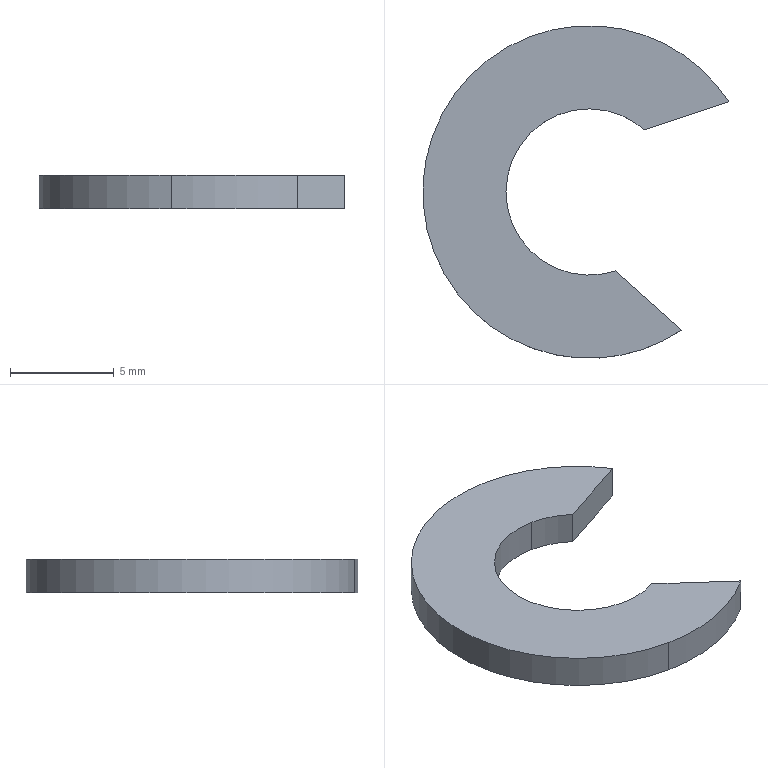Part | NX | features BREP 1 | 1 solid | 10 faces | box 14.725 x 16 x 1.6 mm | volume 174.89 mm3 | cylinder 6 | plane 4 | commonest cylinder face diameters 8 x3 16 x3
STEP:
#1=CARTESIAN_POINT('',(-88.551,270.656,26.6));
#2=VERTEX_POINT('',#1);
#3=CARTESIAN_POINT('',(-91.791,254.987,26.6));
#4=VERTEX_POINT('',#3);
#5=CARTESIAN_POINT('',(-90.171,262.821,26.6));
#6=DIRECTION('',(0.,0.,1.));
#7=DIRECTION('',(0.2024,0.9793,0.));
#8=AXIS2_PLACEMENT_3D('',#5,#6,#7);
#9=CIRCLE('',#8,8.);
#10=EDGE_CURVE('',#2,#4,#9,.T.);
#11=ORIENTED_EDGE('',*,*,#10,.F.);
#12=CARTESIAN_POINT('',(-88.551,270.656,25.));
#13=VERTEX_POINT('',#12);
#14=CARTESIAN_POINT('',(-88.551,270.656,26.6));
#15=DIRECTION('',(0.,0.,-1.));
#16=VECTOR('',#15,1000.);
#17=LINE('',#14,#16);
#18=EDGE_CURVE('',#2,#13,#17,.T.);
#19=ORIENTED_EDGE('',*,*,#18,.T.);
#20=CARTESIAN_POINT('',(-91.791,254.987,25.));
#21=VERTEX_POINT('',#20);
#22=CARTESIAN_POINT('',(-90.171,262.821,25.));
#23=DIRECTION('',(0.,0.,1.));
#24=DIRECTION('',(0.2024,0.9793,0.));
#25=AXIS2_PLACEMENT_3D('',#22,#23,#24);
#26=CIRCLE('',#25,8.);
#27=EDGE_CURVE('',#13,#21,#26,.T.);
#28=ORIENTED_EDGE('',*,*,#27,.T.);
#29=CARTESIAN_POINT('',(-91.791,254.987,26.6));
#30=DIRECTION('',(0.,0.,-1.));
#31=VECTOR('',#30,1000.);
#32=LINE('',#29,#31);
#33=EDGE_CURVE('',#4,#21,#32,.T.);
#34=ORIENTED_EDGE('',*,*,#33,.F.);
#35=EDGE_LOOP('',(#11,#19,#28,#34));
#36=FACE_BOUND('',#35,.T.);
#37=CARTESIAN_POINT('',(-90.171,262.821,26.6));
#38=DIRECTION('',(0.,0.,-1.));
#39=DIRECTION('',(0.2024,0.9793,0.));
#40=AXIS2_PLACEMENT_3D('',#37,#38,#39);
#41=CYLINDRICAL_SURFACE('',#40,8.);
#42=ADVANCED_FACE('',(#36),#41,.T.);
#43=CARTESIAN_POINT('',(-85.716,256.177,26.6));
#44=VERTEX_POINT('',#43);
#45=CARTESIAN_POINT('',(-90.171,262.821,26.6));
#46=DIRECTION('',(0.,0.,1.));
#47=DIRECTION('',(0.2024,0.9793,0.));
#48=AXIS2_PLACEMENT_3D('',#45,#46,#47);
#49=CIRCLE('',#48,8.);
#50=EDGE_CURVE('',#4,#44,#49,.T.);
#51=ORIENTED_EDGE('',*,*,#50,.F.);
#52=ORIENTED_EDGE('',*,*,#33,.T.);
#53=CARTESIAN_POINT('',(-85.716,256.177,25.));
#54=VERTEX_POINT('',#53);
#55=CARTESIAN_POINT('',(-90.171,262.821,25.));
#56=DIRECTION('',(0.,0.,1.));
#57=DIRECTION('',(0.2024,0.9793,0.));
#58=AXIS2_PLACEMENT_3D('',#55,#56,#57);
#59=CIRCLE('',#58,8.);
#60=EDGE_CURVE('',#21,#54,#59,.T.);
#61=ORIENTED_EDGE('',*,*,#60,.T.);
#62=CARTESIAN_POINT('',(-85.716,256.177,26.6));
#63=DIRECTION('',(0.,0.,-1.));
#64=VECTOR('',#63,1000.);
#65=LINE('',#62,#64);
#66=EDGE_CURVE('',#44,#54,#65,.T.);
#67=ORIENTED_EDGE('',*,*,#66,.F.);
#68=EDGE_LOOP('',(#51,#52,#61,#67));
#69=FACE_BOUND('',#68,.T.);
#70=CARTESIAN_POINT('',(-90.171,262.821,26.6));
#71=DIRECTION('',(0.,0.,-1.));
#72=DIRECTION('',(0.2024,0.9793,0.));
#73=AXIS2_PLACEMENT_3D('',#70,#71,#72);
#74=CYLINDRICAL_SURFACE('',#73,8.);
#75=ADVANCED_FACE('',(#69),#74,.T.);
#76=CARTESIAN_POINT('',(-89.361,266.739,26.6));
#77=VERTEX_POINT('',#76);
#78=CARTESIAN_POINT('',(-87.511,265.809,26.6));
#79=VERTEX_POINT('',#78);
#80=CARTESIAN_POINT('',(-90.171,262.821,26.6));
#81=DIRECTION('',(0.,0.,-1.));
#82=DIRECTION('',(0.2024,0.9793,0.));
#83=AXIS2_PLACEMENT_3D('',#80,#81,#82);
#84=CIRCLE('',#83,4.);
#85=EDGE_CURVE('',#77,#79,#84,.T.);
#86=ORIENTED_EDGE('',*,*,#85,.F.);
#87=CARTESIAN_POINT('',(-89.361,266.739,25.));
#88=VERTEX_POINT('',#87);
#89=CARTESIAN_POINT('',(-89.361,266.739,26.6));
#90=DIRECTION('',(0.,0.,-1.));
#91=VECTOR('',#90,1000.);
#92=LINE('',#89,#91);
#93=EDGE_CURVE('',#77,#88,#92,.T.);
#94=ORIENTED_EDGE('',*,*,#93,.T.);
#95=CARTESIAN_POINT('',(-87.511,265.809,25.));
#96=VERTEX_POINT('',#95);
#97=CARTESIAN_POINT('',(-90.171,262.821,25.));
#98=DIRECTION('',(0.,0.,-1.));
#99=DIRECTION('',(0.2024,0.9793,0.));
#100=AXIS2_PLACEMENT_3D('',#97,#98,#99);
#101=CIRCLE('',#100,4.);
#102=EDGE_CURVE('',#88,#96,#101,.T.);
#103=ORIENTED_EDGE('',*,*,#102,.T.);
#104=CARTESIAN_POINT('',(-87.511,265.809,26.6));
#105=DIRECTION('',(0.,0.,-1.));
#106=VECTOR('',#105,1000.);
#107=LINE('',#104,#106);
#108=EDGE_CURVE('',#79,#96,#107,.T.);
#109=ORIENTED_EDGE('',*,*,#108,.F.);
#110=EDGE_LOOP('',(#86,#94,#103,#109));
#111=FACE_BOUND('',#110,.T.);
#112=CARTESIAN_POINT('',(-90.171,262.821,26.6));
#113=DIRECTION('',(0.,0.,-1.));
#114=DIRECTION('',(0.2024,0.9793,0.));
#115=AXIS2_PLACEMENT_3D('',#112,#113,#114);
#116=CYLINDRICAL_SURFACE('',#115,4.);
#117=ADVANCED_FACE('',(#111),#116,.F.);
#118=ORIENTED_EDGE('',*,*,#93,.F.);
#119=CARTESIAN_POINT('',(-90.981,258.904,26.6));
#120=VERTEX_POINT('',#119);
#121=CARTESIAN_POINT('',(-90.171,262.821,26.6));
#122=DIRECTION('',(0.,0.,-1.));
#123=DIRECTION('',(0.2024,0.9793,0.));
#124=AXIS2_PLACEMENT_3D('',#121,#122,#123);
#125=CIRCLE('',#124,4.);
#126=EDGE_CURVE('',#120,#77,#125,.T.);
#127=ORIENTED_EDGE('',*,*,#126,.F.);
#128=CARTESIAN_POINT('',(-90.981,258.904,25.));
#129=VERTEX_POINT('',#128);
#130=CARTESIAN_POINT('',(-90.981,258.904,26.6));
#131=DIRECTION('',(0.,0.,-1.));
#132=VECTOR('',#131,1000.);
#133=LINE('',#130,#132);
#134=EDGE_CURVE('',#120,#129,#133,.T.);
#135=ORIENTED_EDGE('',*,*,#134,.T.);
#136=CARTESIAN_POINT('',(-90.171,262.821,25.));
#137=DIRECTION('',(0.,0.,-1.));
#138=DIRECTION('',(0.2024,0.9793,0.));
#139=AXIS2_PLACEMENT_3D('',#136,#137,#138);
#140=CIRCLE('',#139,4.);
#141=EDGE_CURVE('',#129,#88,#140,.T.);
#142=ORIENTED_EDGE('',*,*,#141,.T.);
#143=EDGE_LOOP('',(#118,#127,#135,#142));
#144=FACE_BOUND('',#143,.T.);
#145=CARTESIAN_POINT('',(-90.171,262.821,26.6));
#146=DIRECTION('',(0.,0.,-1.));
#147=DIRECTION('',(0.2024,0.9793,0.));
#148=AXIS2_PLACEMENT_3D('',#145,#146,#147);
#149=CYLINDRICAL_SURFACE('',#148,4.);
#150=ADVANCED_FACE('',(#144),#149,.F.);
#151=ORIENTED_EDGE('',*,*,#134,.F.);
#152=CARTESIAN_POINT('',(-88.914,259.024,26.6));
#153=VERTEX_POINT('',#152);
#154=CARTESIAN_POINT('',(-90.171,262.821,26.6));
#155=DIRECTION('',(0.,0.,-1.));
#156=DIRECTION('',(0.2024,0.9793,0.));
#157=AXIS2_PLACEMENT_3D('',#154,#155,#156);
#158=CIRCLE('',#157,4.);
#159=EDGE_CURVE('',#153,#120,#158,.T.);
#160=ORIENTED_EDGE('',*,*,#159,.F.);
#161=CARTESIAN_POINT('',(-88.914,259.024,25.));
#162=VERTEX_POINT('',#161);
#163=CARTESIAN_POINT('',(-88.914,259.024,26.6));
#164=DIRECTION('',(0.,0.,-1.));
#165=VECTOR('',#164,1000.);
#166=LINE('',#163,#165);
#167=EDGE_CURVE('',#153,#162,#166,.T.);
#168=ORIENTED_EDGE('',*,*,#167,.T.);
#169=CARTESIAN_POINT('',(-90.171,262.821,25.));
#170=DIRECTION('',(0.,0.,-1.));
#171=DIRECTION('',(0.2024,0.9793,0.));
#172=AXIS2_PLACEMENT_3D('',#169,#170,#171);
#173=CIRCLE('',#172,4.);
#174=EDGE_CURVE('',#162,#129,#173,.T.);
#175=ORIENTED_EDGE('',*,*,#174,.T.);
#176=EDGE_LOOP('',(#151,#160,#168,#175));
#177=FACE_BOUND('',#176,.T.);
#178=CARTESIAN_POINT('',(-90.171,262.821,26.6));
#179=DIRECTION('',(0.,0.,-1.));
#180=DIRECTION('',(0.2024,0.9793,0.));
#181=AXIS2_PLACEMENT_3D('',#178,#179,#180);
#182=CYLINDRICAL_SURFACE('',#181,4.);
#183=ADVANCED_FACE('',(#177),#182,.F.);
#184=CARTESIAN_POINT('',(-83.446,267.155,25.));
#185=VERTEX_POINT('',#184);
#186=CARTESIAN_POINT('',(-87.511,265.809,25.));
#187=DIRECTION('',(0.9493,0.3143,0.));
#188=VECTOR('',#187,1000.);
#189=LINE('',#186,#188);
#190=EDGE_CURVE('',#96,#185,#189,.T.);
#191=ORIENTED_EDGE('',*,*,#190,.T.);
#192=CARTESIAN_POINT('',(-83.446,267.155,26.6));
#193=VERTEX_POINT('',#192);
#194=CARTESIAN_POINT('',(-83.446,267.155,26.6));
#195=DIRECTION('',(0.,0.,-1.));
#196=VECTOR('',#195,1000.);
#197=LINE('',#194,#196);
#198=EDGE_CURVE('',#193,#185,#197,.T.);
#199=ORIENTED_EDGE('',*,*,#198,.F.);
#200=CARTESIAN_POINT('',(-87.511,265.809,26.6));
#201=DIRECTION('',(0.9493,0.3143,0.));
#202=VECTOR('',#201,1000.);
#203=LINE('',#200,#202);
#204=EDGE_CURVE('',#79,#193,#203,.T.);
#205=ORIENTED_EDGE('',*,*,#204,.F.);
#206=ORIENTED_EDGE('',*,*,#108,.T.);
#207=EDGE_LOOP('',(#191,#199,#205,#206));
#208=FACE_BOUND('',#207,.T.);
#209=CARTESIAN_POINT('',(-87.511,265.809,26.6));
#210=DIRECTION('',(-0.3143,0.9493,0.));
#211=DIRECTION('',(0.9493,0.3143,0.));
#212=AXIS2_PLACEMENT_3D('',#209,#210,#211);
#213=PLANE('',#212);
#214=ADVANCED_FACE('',(#208),#213,.F.);
#215=ORIENTED_EDGE('',*,*,#18,.F.);
#216=CARTESIAN_POINT('',(-90.171,262.821,26.6));
#217=DIRECTION('',(0.,0.,1.));
#218=DIRECTION('',(0.2024,0.9793,0.));
#219=AXIS2_PLACEMENT_3D('',#216,#217,#218);
#220=CIRCLE('',#219,8.);
#221=EDGE_CURVE('',#193,#2,#220,.T.);
#222=ORIENTED_EDGE('',*,*,#221,.F.);
#223=ORIENTED_EDGE('',*,*,#198,.T.);
#224=CARTESIAN_POINT('',(-90.171,262.821,25.));
#225=DIRECTION('',(0.,0.,1.));
#226=DIRECTION('',(0.2024,0.9793,0.));
#227=AXIS2_PLACEMENT_3D('',#224,#225,#226);
#228=CIRCLE('',#227,8.);
#229=EDGE_CURVE('',#185,#13,#228,.T.);
#230=ORIENTED_EDGE('',*,*,#229,.T.);
#231=EDGE_LOOP('',(#215,#222,#223,#230));
#232=FACE_BOUND('',#231,.T.);
#233=CARTESIAN_POINT('',(-90.171,262.821,26.6));
#234=DIRECTION('',(0.,0.,-1.));
#235=DIRECTION('',(0.2024,0.9793,0.));
#236=AXIS2_PLACEMENT_3D('',#233,#234,#235);
#237=CYLINDRICAL_SURFACE('',#236,8.);
#238=ADVANCED_FACE('',(#232),#237,.T.);
#239=CARTESIAN_POINT('',(-88.914,259.024,25.));
#240=DIRECTION('',(-0.7469,0.665,0.));
#241=VECTOR('',#240,1000.);
#242=LINE('',#239,#241);
#243=EDGE_CURVE('',#54,#162,#242,.T.);
#244=ORIENTED_EDGE('',*,*,#243,.T.);
#245=ORIENTED_EDGE('',*,*,#167,.F.);
#246=CARTESIAN_POINT('',(-88.914,259.024,26.6));
#247=DIRECTION('',(-0.7469,0.665,0.));
#248=VECTOR('',#247,1000.);
#249=LINE('',#246,#248);
#250=EDGE_CURVE('',#44,#153,#249,.T.);
#251=ORIENTED_EDGE('',*,*,#250,.F.);
#252=ORIENTED_EDGE('',*,*,#66,.T.);
#253=EDGE_LOOP('',(#244,#245,#251,#252));
#254=FACE_BOUND('',#253,.T.);
#255=CARTESIAN_POINT('',(-88.914,259.024,26.6));
#256=DIRECTION('',(-0.665,-0.7469,0.));
#257=DIRECTION('',(-0.7469,0.665,0.));
#258=AXIS2_PLACEMENT_3D('',#255,#256,#257);
#259=PLANE('',#258);
#260=ADVANCED_FACE('',(#254),#259,.F.);
#261=ORIENTED_EDGE('',*,*,#159,.T.);
#262=ORIENTED_EDGE('',*,*,#126,.T.);
#263=ORIENTED_EDGE('',*,*,#85,.T.);
#264=ORIENTED_EDGE('',*,*,#204,.T.);
#265=ORIENTED_EDGE('',*,*,#221,.T.);
#266=ORIENTED_EDGE('',*,*,#10,.T.);
#267=ORIENTED_EDGE('',*,*,#50,.T.);
#268=ORIENTED_EDGE('',*,*,#250,.T.);
#269=EDGE_LOOP('',(#261,#262,#263,#264,#265,#266,#267,#268));
#270=FACE_BOUND('',#269,.T.);
#271=CARTESIAN_POINT('',(-90.171,262.821,26.6));
#272=DIRECTION('',(0.,0.,1.));
#273=DIRECTION('',(-0.2024,-0.9793,0.));
#274=AXIS2_PLACEMENT_3D('',#271,#272,#273);
#275=PLANE('',#274);
#276=ADVANCED_FACE('',(#270),#275,.T.);
#277=ORIENTED_EDGE('',*,*,#174,.F.);
#278=ORIENTED_EDGE('',*,*,#243,.F.);
#279=ORIENTED_EDGE('',*,*,#60,.F.);
#280=ORIENTED_EDGE('',*,*,#27,.F.);
#281=ORIENTED_EDGE('',*,*,#229,.F.);
#282=ORIENTED_EDGE('',*,*,#190,.F.);
#283=ORIENTED_EDGE('',*,*,#102,.F.);
#284=ORIENTED_EDGE('',*,*,#141,.F.);
#285=EDGE_LOOP('',(#277,#278,#279,#280,#281,#282,#283,#284));
#286=FACE_BOUND('',#285,.T.);
#287=CARTESIAN_POINT('',(-90.171,262.821,25.));
#288=DIRECTION('',(0.,0.,1.));
#289=DIRECTION('',(-0.2024,-0.9793,0.));
#290=AXIS2_PLACEMENT_3D('',#287,#288,#289);
#291=PLANE('',#290);
#292=ADVANCED_FACE('',(#286),#291,.F.);
#293=CLOSED_SHELL('',(#42,#75,#117,#150,#183,#214,#238,#260,#276,#292));
#294=MANIFOLD_SOLID_BREP('',#293);
#295=(LENGTH_UNIT()NAMED_UNIT(*)SI_UNIT(.MILLI.,.METRE.));
#296=UNCERTAINTY_MEASURE_WITH_UNIT(LENGTH_MEASURE(0.00001),#295,'','');
#297=(NAMED_UNIT(*)PLANE_ANGLE_UNIT()SI_UNIT($,.RADIAN.));
#298=(NAMED_UNIT(*)SI_UNIT($,.STERADIAN.)SOLID_ANGLE_UNIT());
#299=(GEOMETRIC_REPRESENTATION_CONTEXT(3)GLOBAL_UNCERTAINTY_ASSIGNED_CONTEXT((#296))GLOBAL_UNIT_ASSIGNED_CONTEXT((#295,#297,#298))REPRESENTATION_CONTEXT('',''));
#300=ADVANCED_BREP_SHAPE_REPRESENTATION('',(#294),#299);